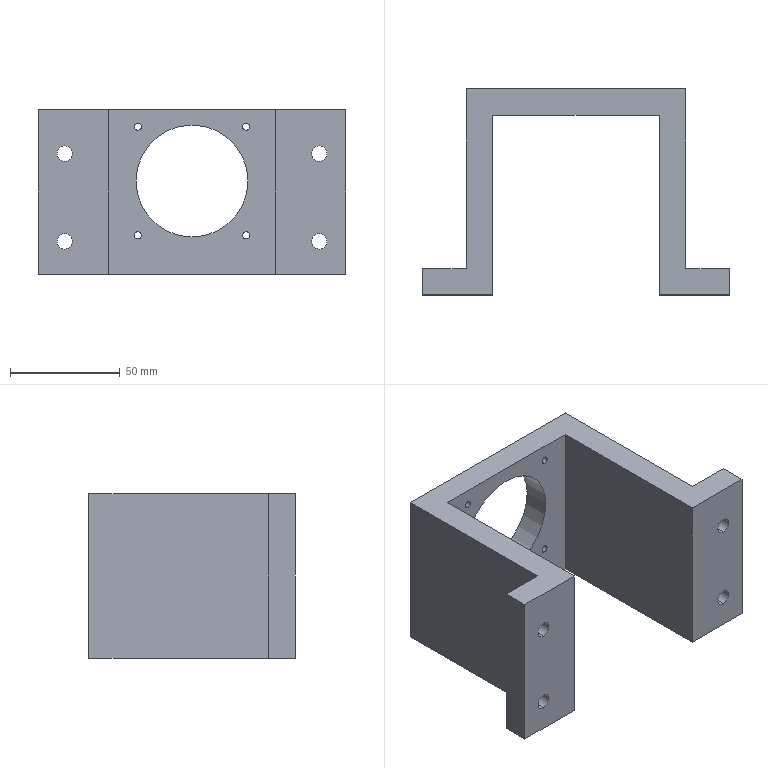Part | SolidWorks | features ICE 2, ExtruThin 1, HoleWzd 1 | 1 solid | 32 faces | box 140 x 94 x 75 mm | volume 246828 mm3 | cylinder 18 | plane 14 | commonest cylinder face diameters 3.3 x8 7 x8 51 x2
STEP:
#1=CARTESIAN_POINT('',(-24.749,70.,16.101));
#2=VERTEX_POINT('',#1);
#3=CARTESIAN_POINT('',(-24.749,70.,19.401));
#4=VERTEX_POINT('',#3);
#5=CARTESIAN_POINT('',(-24.749,70.,17.751));
#6=DIRECTION('',(0.,1.,0.));
#7=DIRECTION('',(0.,0.,1.));
#8=AXIS2_PLACEMENT_3D('',#5,#6,#7);
#9=CIRCLE('',#8,1.65);
#10=EDGE_CURVE('',#2,#4,#9,.T.);
#11=ORIENTED_EDGE('',*,*,#10,.F.);
#12=CARTESIAN_POINT('',(-24.749,82.,16.101));
#13=VERTEX_POINT('',#12);
#14=CARTESIAN_POINT('',(-24.749,82.,16.101));
#15=DIRECTION('',(0.,1.,0.));
#16=VECTOR('',#15,1000.);
#17=LINE('',#14,#16);
#18=EDGE_CURVE('',#2,#13,#17,.T.);
#19=ORIENTED_EDGE('',*,*,#18,.T.);
#20=CARTESIAN_POINT('',(-24.749,82.,19.401));
#21=VERTEX_POINT('',#20);
#22=CARTESIAN_POINT('',(-24.749,82.,17.751));
#23=DIRECTION('',(0.,1.,0.));
#24=DIRECTION('',(0.,0.,1.));
#25=AXIS2_PLACEMENT_3D('',#22,#23,#24);
#26=CIRCLE('',#25,1.65);
#27=EDGE_CURVE('',#13,#21,#26,.T.);
#28=ORIENTED_EDGE('',*,*,#27,.T.);
#29=CARTESIAN_POINT('',(-24.749,82.,19.401));
#30=DIRECTION('',(0.,1.,0.));
#31=VECTOR('',#30,1000.);
#32=LINE('',#29,#31);
#33=EDGE_CURVE('',#4,#21,#32,.T.);
#34=ORIENTED_EDGE('',*,*,#33,.F.);
#35=EDGE_LOOP('',(#11,#19,#28,#34));
#36=FACE_OUTER_BOUND('',#35,.T.);
#37=CARTESIAN_POINT('',(-24.749,82.,17.751));
#38=DIRECTION('',(0.,1.,0.));
#39=DIRECTION('',(0.,0.,1.));
#40=AXIS2_PLACEMENT_3D('',#37,#38,#39);
#41=CYLINDRICAL_SURFACE('',#40,1.65);
#42=ADVANCED_FACE('',(#36),#41,.F.);
#43=CARTESIAN_POINT('',(24.749,70.,16.101));
#44=VERTEX_POINT('',#43);
#45=CARTESIAN_POINT('',(24.749,70.,19.401));
#46=VERTEX_POINT('',#45);
#47=CARTESIAN_POINT('',(24.749,70.,17.751));
#48=DIRECTION('',(0.,1.,0.));
#49=DIRECTION('',(0.,0.,1.));
#50=AXIS2_PLACEMENT_3D('',#47,#48,#49);
#51=CIRCLE('',#50,1.65);
#52=EDGE_CURVE('',#44,#46,#51,.T.);
#53=ORIENTED_EDGE('',*,*,#52,.F.);
#54=CARTESIAN_POINT('',(24.749,82.,16.101));
#55=VERTEX_POINT('',#54);
#56=CARTESIAN_POINT('',(24.749,82.,16.101));
#57=DIRECTION('',(0.,1.,0.));
#58=VECTOR('',#57,1000.);
#59=LINE('',#56,#58);
#60=EDGE_CURVE('',#44,#55,#59,.T.);
#61=ORIENTED_EDGE('',*,*,#60,.T.);
#62=CARTESIAN_POINT('',(24.749,82.,19.401));
#63=VERTEX_POINT('',#62);
#64=CARTESIAN_POINT('',(24.749,82.,17.751));
#65=DIRECTION('',(0.,1.,0.));
#66=DIRECTION('',(0.,0.,1.));
#67=AXIS2_PLACEMENT_3D('',#64,#65,#66);
#68=CIRCLE('',#67,1.65);
#69=EDGE_CURVE('',#55,#63,#68,.T.);
#70=ORIENTED_EDGE('',*,*,#69,.T.);
#71=CARTESIAN_POINT('',(24.749,82.,19.401));
#72=DIRECTION('',(0.,1.,0.));
#73=VECTOR('',#72,1000.);
#74=LINE('',#71,#73);
#75=EDGE_CURVE('',#46,#63,#74,.T.);
#76=ORIENTED_EDGE('',*,*,#75,.F.);
#77=EDGE_LOOP('',(#53,#61,#70,#76));
#78=FACE_OUTER_BOUND('',#77,.T.);
#79=CARTESIAN_POINT('',(24.749,82.,17.751));
#80=DIRECTION('',(0.,1.,0.));
#81=DIRECTION('',(0.,0.,1.));
#82=AXIS2_PLACEMENT_3D('',#79,#80,#81);
#83=CYLINDRICAL_SURFACE('',#82,1.65);
#84=ADVANCED_FACE('',(#78),#83,.F.);
#85=CARTESIAN_POINT('',(24.749,70.,65.599));
#86=VERTEX_POINT('',#85);
#87=CARTESIAN_POINT('',(24.749,70.,68.899));
#88=VERTEX_POINT('',#87);
#89=CARTESIAN_POINT('',(24.749,70.,67.249));
#90=DIRECTION('',(0.,1.,0.));
#91=DIRECTION('',(0.,0.,1.));
#92=AXIS2_PLACEMENT_3D('',#89,#90,#91);
#93=CIRCLE('',#92,1.65);
#94=EDGE_CURVE('',#86,#88,#93,.T.);
#95=ORIENTED_EDGE('',*,*,#94,.F.);
#96=CARTESIAN_POINT('',(24.749,82.,65.599));
#97=VERTEX_POINT('',#96);
#98=CARTESIAN_POINT('',(24.749,82.,65.599));
#99=DIRECTION('',(0.,1.,0.));
#100=VECTOR('',#99,1000.);
#101=LINE('',#98,#100);
#102=EDGE_CURVE('',#86,#97,#101,.T.);
#103=ORIENTED_EDGE('',*,*,#102,.T.);
#104=CARTESIAN_POINT('',(24.749,82.,68.899));
#105=VERTEX_POINT('',#104);
#106=CARTESIAN_POINT('',(24.749,82.,67.249));
#107=DIRECTION('',(0.,1.,0.));
#108=DIRECTION('',(0.,0.,1.));
#109=AXIS2_PLACEMENT_3D('',#106,#107,#108);
#110=CIRCLE('',#109,1.65);
#111=EDGE_CURVE('',#97,#105,#110,.T.);
#112=ORIENTED_EDGE('',*,*,#111,.T.);
#113=CARTESIAN_POINT('',(24.749,82.,68.899));
#114=DIRECTION('',(0.,1.,0.));
#115=VECTOR('',#114,1000.);
#116=LINE('',#113,#115);
#117=EDGE_CURVE('',#88,#105,#116,.T.);
#118=ORIENTED_EDGE('',*,*,#117,.F.);
#119=EDGE_LOOP('',(#95,#103,#112,#118));
#120=FACE_OUTER_BOUND('',#119,.T.);
#121=CARTESIAN_POINT('',(24.749,82.,67.249));
#122=DIRECTION('',(0.,1.,0.));
#123=DIRECTION('',(0.,0.,1.));
#124=AXIS2_PLACEMENT_3D('',#121,#122,#123);
#125=CYLINDRICAL_SURFACE('',#124,1.65);
#126=ADVANCED_FACE('',(#120),#125,.F.);
#127=CARTESIAN_POINT('',(-24.749,70.,65.599));
#128=VERTEX_POINT('',#127);
#129=CARTESIAN_POINT('',(-24.749,70.,68.899));
#130=VERTEX_POINT('',#129);
#131=CARTESIAN_POINT('',(-24.749,70.,67.249));
#132=DIRECTION('',(0.,1.,0.));
#133=DIRECTION('',(0.,0.,1.));
#134=AXIS2_PLACEMENT_3D('',#131,#132,#133);
#135=CIRCLE('',#134,1.65);
#136=EDGE_CURVE('',#128,#130,#135,.T.);
#137=ORIENTED_EDGE('',*,*,#136,.F.);
#138=CARTESIAN_POINT('',(-24.749,82.,65.599));
#139=VERTEX_POINT('',#138);
#140=CARTESIAN_POINT('',(-24.749,82.,65.599));
#141=DIRECTION('',(0.,1.,0.));
#142=VECTOR('',#141,1000.);
#143=LINE('',#140,#142);
#144=EDGE_CURVE('',#128,#139,#143,.T.);
#145=ORIENTED_EDGE('',*,*,#144,.T.);
#146=CARTESIAN_POINT('',(-24.749,82.,68.899));
#147=VERTEX_POINT('',#146);
#148=CARTESIAN_POINT('',(-24.749,82.,67.249));
#149=DIRECTION('',(0.,1.,0.));
#150=DIRECTION('',(0.,0.,1.));
#151=AXIS2_PLACEMENT_3D('',#148,#149,#150);
#152=CIRCLE('',#151,1.65);
#153=EDGE_CURVE('',#139,#147,#152,.T.);
#154=ORIENTED_EDGE('',*,*,#153,.T.);
#155=CARTESIAN_POINT('',(-24.749,82.,68.899));
#156=DIRECTION('',(0.,1.,0.));
#157=VECTOR('',#156,1000.);
#158=LINE('',#155,#157);
#159=EDGE_CURVE('',#130,#147,#158,.T.);
#160=ORIENTED_EDGE('',*,*,#159,.F.);
#161=EDGE_LOOP('',(#137,#145,#154,#160));
#162=FACE_OUTER_BOUND('',#161,.T.);
#163=CARTESIAN_POINT('',(-24.749,82.,67.249));
#164=DIRECTION('',(0.,1.,0.));
#165=DIRECTION('',(0.,0.,1.));
#166=AXIS2_PLACEMENT_3D('',#163,#164,#165);
#167=CYLINDRICAL_SURFACE('',#166,1.65);
#168=ADVANCED_FACE('',(#162),#167,.F.);
#169=CARTESIAN_POINT('',(-58.,-12.,51.5));
#170=VERTEX_POINT('',#169);
#171=CARTESIAN_POINT('',(-58.,-12.,58.5));
#172=VERTEX_POINT('',#171);
#173=CARTESIAN_POINT('',(-58.,-12.,55.));
#174=DIRECTION('',(0.,1.,0.));
#175=DIRECTION('',(0.,0.,-1.));
#176=AXIS2_PLACEMENT_3D('',#173,#174,#175);
#177=CIRCLE('',#176,3.5);
#178=EDGE_CURVE('',#170,#172,#177,.T.);
#179=ORIENTED_EDGE('',*,*,#178,.F.);
#180=CARTESIAN_POINT('',(-58.,0.,51.5));
#181=VERTEX_POINT('',#180);
#182=CARTESIAN_POINT('',(-58.,-12.,51.5));
#183=DIRECTION('',(0.,1.,0.));
#184=VECTOR('',#183,1000.);
#185=LINE('',#182,#184);
#186=EDGE_CURVE('',#170,#181,#185,.T.);
#187=ORIENTED_EDGE('',*,*,#186,.T.);
#188=CARTESIAN_POINT('',(-58.,0.,58.5));
#189=VERTEX_POINT('',#188);
#190=CARTESIAN_POINT('',(-58.,0.,55.));
#191=DIRECTION('',(0.,1.,0.));
#192=DIRECTION('',(0.,0.,-1.));
#193=AXIS2_PLACEMENT_3D('',#190,#191,#192);
#194=CIRCLE('',#193,3.5);
#195=EDGE_CURVE('',#181,#189,#194,.T.);
#196=ORIENTED_EDGE('',*,*,#195,.T.);
#197=CARTESIAN_POINT('',(-58.,-12.,58.5));
#198=DIRECTION('',(0.,1.,0.));
#199=VECTOR('',#198,1000.);
#200=LINE('',#197,#199);
#201=EDGE_CURVE('',#172,#189,#200,.T.);
#202=ORIENTED_EDGE('',*,*,#201,.F.);
#203=EDGE_LOOP('',(#179,#187,#196,#202));
#204=FACE_OUTER_BOUND('',#203,.T.);
#205=CARTESIAN_POINT('',(-58.,-12.,55.));
#206=DIRECTION('',(0.,1.,0.));
#207=DIRECTION('',(0.,0.,1.));
#208=AXIS2_PLACEMENT_3D('',#205,#206,#207);
#209=CYLINDRICAL_SURFACE('',#208,3.5);
#210=ADVANCED_FACE('',(#204),#209,.F.);
#211=CARTESIAN_POINT('',(58.,-12.,51.5));
#212=VERTEX_POINT('',#211);
#213=CARTESIAN_POINT('',(58.,-12.,58.5));
#214=VERTEX_POINT('',#213);
#215=CARTESIAN_POINT('',(58.,-12.,55.));
#216=DIRECTION('',(0.,1.,0.));
#217=DIRECTION('',(0.,0.,1.));
#218=AXIS2_PLACEMENT_3D('',#215,#216,#217);
#219=CIRCLE('',#218,3.5);
#220=EDGE_CURVE('',#212,#214,#219,.T.);
#221=ORIENTED_EDGE('',*,*,#220,.F.);
#222=CARTESIAN_POINT('',(58.,0.,51.5));
#223=VERTEX_POINT('',#222);
#224=CARTESIAN_POINT('',(58.,-12.,51.5));
#225=DIRECTION('',(0.,1.,0.));
#226=VECTOR('',#225,1000.);
#227=LINE('',#224,#226);
#228=EDGE_CURVE('',#212,#223,#227,.T.);
#229=ORIENTED_EDGE('',*,*,#228,.T.);
#230=CARTESIAN_POINT('',(58.,0.,58.5));
#231=VERTEX_POINT('',#230);
#232=CARTESIAN_POINT('',(58.,0.,55.));
#233=DIRECTION('',(0.,1.,0.));
#234=DIRECTION('',(0.,0.,1.));
#235=AXIS2_PLACEMENT_3D('',#232,#233,#234);
#236=CIRCLE('',#235,3.5);
#237=EDGE_CURVE('',#223,#231,#236,.T.);
#238=ORIENTED_EDGE('',*,*,#237,.T.);
#239=CARTESIAN_POINT('',(58.,-12.,58.5));
#240=DIRECTION('',(0.,1.,0.));
#241=VECTOR('',#240,1000.);
#242=LINE('',#239,#241);
#243=EDGE_CURVE('',#214,#231,#242,.T.);
#244=ORIENTED_EDGE('',*,*,#243,.F.);
#245=EDGE_LOOP('',(#221,#229,#238,#244));
#246=FACE_OUTER_BOUND('',#245,.T.);
#247=CARTESIAN_POINT('',(58.,-12.,55.));
#248=DIRECTION('',(0.,1.,0.));
#249=DIRECTION('',(0.,0.,1.));
#250=AXIS2_PLACEMENT_3D('',#247,#248,#249);
#251=CYLINDRICAL_SURFACE('',#250,3.5);
#252=ADVANCED_FACE('',(#246),#251,.F.);
#253=CARTESIAN_POINT('',(58.,-12.,11.5));
#254=VERTEX_POINT('',#253);
#255=CARTESIAN_POINT('',(58.,-12.,18.5));
#256=VERTEX_POINT('',#255);
#257=CARTESIAN_POINT('',(58.,-12.,15.));
#258=DIRECTION('',(0.,1.,0.));
#259=DIRECTION('',(0.,0.,-1.));
#260=AXIS2_PLACEMENT_3D('',#257,#258,#259);
#261=CIRCLE('',#260,3.5);
#262=EDGE_CURVE('',#254,#256,#261,.T.);
#263=ORIENTED_EDGE('',*,*,#262,.F.);
#264=CARTESIAN_POINT('',(58.,0.,11.5));
#265=VERTEX_POINT('',#264);
#266=CARTESIAN_POINT('',(58.,-12.,11.5));
#267=DIRECTION('',(0.,1.,0.));
#268=VECTOR('',#267,1000.);
#269=LINE('',#266,#268);
#270=EDGE_CURVE('',#254,#265,#269,.T.);
#271=ORIENTED_EDGE('',*,*,#270,.T.);
#272=CARTESIAN_POINT('',(58.,0.,18.5));
#273=VERTEX_POINT('',#272);
#274=CARTESIAN_POINT('',(58.,0.,15.));
#275=DIRECTION('',(0.,1.,0.));
#276=DIRECTION('',(0.,0.,-1.));
#277=AXIS2_PLACEMENT_3D('',#274,#275,#276);
#278=CIRCLE('',#277,3.5);
#279=EDGE_CURVE('',#265,#273,#278,.T.);
#280=ORIENTED_EDGE('',*,*,#279,.T.);
#281=CARTESIAN_POINT('',(58.,-12.,18.5));
#282=DIRECTION('',(0.,1.,0.));
#283=VECTOR('',#282,1000.);
#284=LINE('',#281,#283);
#285=EDGE_CURVE('',#256,#273,#284,.T.);
#286=ORIENTED_EDGE('',*,*,#285,.F.);
#287=EDGE_LOOP('',(#263,#271,#280,#286));
#288=FACE_OUTER_BOUND('',#287,.T.);
#289=CARTESIAN_POINT('',(58.,-12.,15.));
#290=DIRECTION('',(0.,1.,0.));
#291=DIRECTION('',(0.,0.,1.));
#292=AXIS2_PLACEMENT_3D('',#289,#290,#291);
#293=CYLINDRICAL_SURFACE('',#292,3.5);
#294=ADVANCED_FACE('',(#288),#293,.F.);
#295=CARTESIAN_POINT('',(-58.,-12.,11.5));
#296=VERTEX_POINT('',#295);
#297=CARTESIAN_POINT('',(-58.,-12.,18.5));
#298=VERTEX_POINT('',#297);
#299=CARTESIAN_POINT('',(-58.,-12.,15.));
#300=DIRECTION('',(0.,1.,0.));
#301=DIRECTION('',(0.,0.,1.));
#302=AXIS2_PLACEMENT_3D('',#299,#300,#301);
#303=CIRCLE('',#302,3.5);
#304=EDGE_CURVE('',#296,#298,#303,.T.);
#305=ORIENTED_EDGE('',*,*,#304,.F.);
#306=CARTESIAN_POINT('',(-58.,0.,11.5));
#307=VERTEX_POINT('',#306);
#308=CARTESIAN_POINT('',(-58.,-12.,11.5));
#309=DIRECTION('',(0.,1.,0.));
#310=VECTOR('',#309,1000.);
#311=LINE('',#308,#310);
#312=EDGE_CURVE('',#296,#307,#311,.T.);
#313=ORIENTED_EDGE('',*,*,#312,.T.);
#314=CARTESIAN_POINT('',(-58.,0.,18.5));
#315=VERTEX_POINT('',#314);
#316=CARTESIAN_POINT('',(-58.,0.,15.));
#317=DIRECTION('',(0.,1.,0.));
#318=DIRECTION('',(0.,0.,1.));
#319=AXIS2_PLACEMENT_3D('',#316,#317,#318);
#320=CIRCLE('',#319,3.5);
#321=EDGE_CURVE('',#307,#315,#320,.T.);
#322=ORIENTED_EDGE('',*,*,#321,.T.);
#323=CARTESIAN_POINT('',(-58.,-12.,18.5));
#324=DIRECTION('',(0.,1.,0.));
#325=VECTOR('',#324,1000.);
#326=LINE('',#323,#325);
#327=EDGE_CURVE('',#298,#315,#326,.T.);
#328=ORIENTED_EDGE('',*,*,#327,.F.);
#329=EDGE_LOOP('',(#305,#313,#322,#328));
#330=FACE_OUTER_BOUND('',#329,.T.);
#331=CARTESIAN_POINT('',(-58.,-12.,15.));
#332=DIRECTION('',(0.,1.,0.));
#333=DIRECTION('',(0.,0.,1.));
#334=AXIS2_PLACEMENT_3D('',#331,#332,#333);
#335=CYLINDRICAL_SURFACE('',#334,3.5);
#336=ADVANCED_FACE('',(#330),#335,.F.);
#337=CARTESIAN_POINT('',(0.,70.,17.));
#338=VERTEX_POINT('',#337);
#339=CARTESIAN_POINT('',(0.,70.,68.));
#340=VERTEX_POINT('',#339);
#341=CARTESIAN_POINT('',(0.,70.,42.5));
#342=DIRECTION('',(0.,1.,0.));
#343=DIRECTION('',(0.,0.,1.));
#344=AXIS2_PLACEMENT_3D('',#341,#342,#343);
#345=CIRCLE('',#344,25.5);
#346=EDGE_CURVE('',#338,#340,#345,.T.);
#347=ORIENTED_EDGE('',*,*,#346,.F.);
#348=CARTESIAN_POINT('',(0.,82.,17.));
#349=VERTEX_POINT('',#348);
#350=CARTESIAN_POINT('',(0.,-12.,17.));
#351=DIRECTION('',(0.,1.,0.));
#352=VECTOR('',#351,1000.);
#353=LINE('',#350,#352);
#354=EDGE_CURVE('',#338,#349,#353,.T.);
#355=ORIENTED_EDGE('',*,*,#354,.T.);
#356=CARTESIAN_POINT('',(0.,82.,68.));
#357=VERTEX_POINT('',#356);
#358=CARTESIAN_POINT('',(0.,82.,42.5));
#359=DIRECTION('',(0.,1.,0.));
#360=DIRECTION('',(0.,0.,1.));
#361=AXIS2_PLACEMENT_3D('',#358,#359,#360);
#362=CIRCLE('',#361,25.5);
#363=EDGE_CURVE('',#349,#357,#362,.T.);
#364=ORIENTED_EDGE('',*,*,#363,.T.);
#365=CARTESIAN_POINT('',(0.,-12.,68.));
#366=DIRECTION('',(0.,1.,0.));
#367=VECTOR('',#366,1000.);
#368=LINE('',#365,#367);
#369=EDGE_CURVE('',#340,#357,#368,.T.);
#370=ORIENTED_EDGE('',*,*,#369,.F.);
#371=EDGE_LOOP('',(#347,#355,#364,#370));
#372=FACE_OUTER_BOUND('',#371,.T.);
#373=CARTESIAN_POINT('',(0.,-12.,42.5));
#374=DIRECTION('',(0.,1.,0.));
#375=DIRECTION('',(0.,0.,1.));
#376=AXIS2_PLACEMENT_3D('',#373,#374,#375);
#377=CYLINDRICAL_SURFACE('',#376,25.5);
#378=ADVANCED_FACE('',(#372),#377,.F.);
#379=CARTESIAN_POINT('',(58.,-12.,55.));
#380=DIRECTION('',(0.,1.,0.));
#381=DIRECTION('',(0.,0.,1.));
#382=AXIS2_PLACEMENT_3D('',#379,#380,#381);
#383=CIRCLE('',#382,3.5);
#384=EDGE_CURVE('',#214,#212,#383,.T.);
#385=ORIENTED_EDGE('',*,*,#384,.T.);
#386=ORIENTED_EDGE('',*,*,#220,.T.);
#387=EDGE_LOOP('',(#385,#386));
#388=FACE_BOUND('',#387,.T.);
#389=CARTESIAN_POINT('',(58.,-12.,15.));
#390=DIRECTION('',(0.,1.,0.));
#391=DIRECTION('',(0.,0.,-1.));
#392=AXIS2_PLACEMENT_3D('',#389,#390,#391);
#393=CIRCLE('',#392,3.5);
#394=EDGE_CURVE('',#256,#254,#393,.T.);
#395=ORIENTED_EDGE('',*,*,#394,.T.);
#396=ORIENTED_EDGE('',*,*,#262,.T.);
#397=EDGE_LOOP('',(#395,#396));
#398=FACE_BOUND('',#397,.T.);
#399=CARTESIAN_POINT('',(38.,-12.,0.));
#400=VERTEX_POINT('',#399);
#401=CARTESIAN_POINT('',(70.,-12.,0.));
#402=VERTEX_POINT('',#401);
#403=CARTESIAN_POINT('',(50.,-12.,0.));
#404=DIRECTION('',(1.,0.,0.));
#405=VECTOR('',#404,1000.);
#406=LINE('',#403,#405);
#407=EDGE_CURVE('',#400,#402,#406,.T.);
#408=ORIENTED_EDGE('',*,*,#407,.T.);
#409=CARTESIAN_POINT('',(70.,-12.,75.));
#410=VERTEX_POINT('',#409);
#411=CARTESIAN_POINT('',(70.,-12.,75.));
#412=DIRECTION('',(0.,0.,-1.));
#413=VECTOR('',#412,1000.);
#414=LINE('',#411,#413);
#415=EDGE_CURVE('',#410,#402,#414,.T.);
#416=ORIENTED_EDGE('',*,*,#415,.F.);
#417=CARTESIAN_POINT('',(38.,-12.,75.));
#418=VERTEX_POINT('',#417);
#419=CARTESIAN_POINT('',(50.,-12.,75.));
#420=DIRECTION('',(1.,0.,0.));
#421=VECTOR('',#420,1000.);
#422=LINE('',#419,#421);
#423=EDGE_CURVE('',#418,#410,#422,.T.);
#424=ORIENTED_EDGE('',*,*,#423,.F.);
#425=CARTESIAN_POINT('',(38.,-12.,75.));
#426=DIRECTION('',(0.,0.,-1.));
#427=VECTOR('',#426,1000.);
#428=LINE('',#425,#427);
#429=EDGE_CURVE('',#418,#400,#428,.T.);
#430=ORIENTED_EDGE('',*,*,#429,.T.);
#431=EDGE_LOOP('',(#408,#416,#424,#430));
#432=FACE_OUTER_BOUND('',#431,.T.);
#433=CARTESIAN_POINT('',(50.,-12.,75.));
#434=DIRECTION('',(0.,1.,0.));
#435=DIRECTION('',(0.,0.,1.));
#436=AXIS2_PLACEMENT_3D('',#433,#434,#435);
#437=PLANE('',#436);
#438=ADVANCED_FACE('',(#388,#398,#432),#437,.F.);
#439=CARTESIAN_POINT('',(70.,0.,0.));
#440=VERTEX_POINT('',#439);
#441=CARTESIAN_POINT('',(70.,0.,0.));
#442=DIRECTION('',(0.,-1.,0.));
#443=VECTOR('',#442,1000.);
#444=LINE('',#441,#443);
#445=EDGE_CURVE('',#440,#402,#444,.T.);
#446=ORIENTED_EDGE('',*,*,#445,.F.);
#447=CARTESIAN_POINT('',(70.,0.,75.));
#448=VERTEX_POINT('',#447);
#449=CARTESIAN_POINT('',(70.,0.,75.));
#450=DIRECTION('',(0.,0.,-1.));
#451=VECTOR('',#450,1000.);
#452=LINE('',#449,#451);
#453=EDGE_CURVE('',#448,#440,#452,.T.);
#454=ORIENTED_EDGE('',*,*,#453,.F.);
#455=CARTESIAN_POINT('',(70.,0.,75.));
#456=DIRECTION('',(0.,-1.,0.));
#457=VECTOR('',#456,1000.);
#458=LINE('',#455,#457);
#459=EDGE_CURVE('',#448,#410,#458,.T.);
#460=ORIENTED_EDGE('',*,*,#459,.T.);
#461=ORIENTED_EDGE('',*,*,#415,.T.);
#462=EDGE_LOOP('',(#446,#454,#460,#461));
#463=FACE_OUTER_BOUND('',#462,.T.);
#464=CARTESIAN_POINT('',(70.,0.,75.));
#465=DIRECTION('',(1.,0.,0.));
#466=DIRECTION('',(0.,0.,-1.));
#467=AXIS2_PLACEMENT_3D('',#464,#465,#466);
#468=PLANE('',#467);
#469=ADVANCED_FACE('',(#463),#468,.T.);
#470=CARTESIAN_POINT('',(58.,0.,55.));
#471=DIRECTION('',(0.,1.,0.));
#472=DIRECTION('',(0.,0.,1.));
#473=AXIS2_PLACEMENT_3D('',#470,#471,#472);
#474=CIRCLE('',#473,3.5);
#475=EDGE_CURVE('',#231,#223,#474,.T.);
#476=ORIENTED_EDGE('',*,*,#475,.F.);
#477=ORIENTED_EDGE('',*,*,#237,.F.);
#478=EDGE_LOOP('',(#476,#477));
#479=FACE_BOUND('',#478,.T.);
#480=CARTESIAN_POINT('',(58.,0.,15.));
#481=DIRECTION('',(0.,1.,0.));
#482=DIRECTION('',(0.,0.,-1.));
#483=AXIS2_PLACEMENT_3D('',#480,#481,#482);
#484=CIRCLE('',#483,3.5);
#485=EDGE_CURVE('',#273,#265,#484,.T.);
#486=ORIENTED_EDGE('',*,*,#485,.F.);
#487=ORIENTED_EDGE('',*,*,#279,.F.);
#488=EDGE_LOOP('',(#486,#487));
#489=FACE_BOUND('',#488,.T.);
#490=CARTESIAN_POINT('',(50.,0.,0.));
#491=VERTEX_POINT('',#490);
#492=CARTESIAN_POINT('',(50.,0.,0.));
#493=DIRECTION('',(1.,0.,0.));
#494=VECTOR('',#493,1000.);
#495=LINE('',#492,#494);
#496=EDGE_CURVE('',#491,#440,#495,.T.);
#497=ORIENTED_EDGE('',*,*,#496,.F.);
#498=CARTESIAN_POINT('',(50.,0.,75.));
#499=VERTEX_POINT('',#498);
#500=CARTESIAN_POINT('',(50.,0.,75.));
#501=DIRECTION('',(0.,0.,-1.));
#502=VECTOR('',#501,1000.);
#503=LINE('',#500,#502);
#504=EDGE_CURVE('',#499,#491,#503,.T.);
#505=ORIENTED_EDGE('',*,*,#504,.F.);
#506=CARTESIAN_POINT('',(50.,0.,75.));
#507=DIRECTION('',(1.,0.,0.));
#508=VECTOR('',#507,1000.);
#509=LINE('',#506,#508);
#510=EDGE_CURVE('',#499,#448,#509,.T.);
#511=ORIENTED_EDGE('',*,*,#510,.T.);
#512=ORIENTED_EDGE('',*,*,#453,.T.);
#513=EDGE_LOOP('',(#497,#505,#511,#512));
#514=FACE_OUTER_BOUND('',#513,.T.);
#515=CARTESIAN_POINT('',(50.,0.,75.));
#516=DIRECTION('',(0.,1.,0.));
#517=DIRECTION('',(0.,0.,1.));
#518=AXIS2_PLACEMENT_3D('',#515,#516,#517);
#519=PLANE('',#518);
#520=ADVANCED_FACE('',(#479,#489,#514),#519,.T.);
#521=CARTESIAN_POINT('',(50.,82.,0.));
#522=VERTEX_POINT('',#521);
#523=CARTESIAN_POINT('',(50.,82.,0.));
#524=DIRECTION('',(0.,-1.,0.));
#525=VECTOR('',#524,1000.);
#526=LINE('',#523,#525);
#527=EDGE_CURVE('',#522,#491,#526,.T.);
#528=ORIENTED_EDGE('',*,*,#527,.F.);
#529=CARTESIAN_POINT('',(50.,82.,75.));
#530=VERTEX_POINT('',#529);
#531=CARTESIAN_POINT('',(50.,82.,75.));
#532=DIRECTION('',(0.,0.,-1.));
#533=VECTOR('',#532,1000.);
#534=LINE('',#531,#533);
#535=EDGE_CURVE('',#530,#522,#534,.T.);
#536=ORIENTED_EDGE('',*,*,#535,.F.);
#537=CARTESIAN_POINT('',(50.,82.,75.));
#538=DIRECTION('',(0.,-1.,0.));
#539=VECTOR('',#538,1000.);
#540=LINE('',#537,#539);
#541=EDGE_CURVE('',#530,#499,#540,.T.);
#542=ORIENTED_EDGE('',*,*,#541,.T.);
#543=ORIENTED_EDGE('',*,*,#504,.T.);
#544=EDGE_LOOP('',(#528,#536,#542,#543));
#545=FACE_OUTER_BOUND('',#544,.T.);
#546=CARTESIAN_POINT('',(50.,82.,75.));
#547=DIRECTION('',(1.,0.,0.));
#548=DIRECTION('',(0.,0.,-1.));
#549=AXIS2_PLACEMENT_3D('',#546,#547,#548);
#550=PLANE('',#549);
#551=ADVANCED_FACE('',(#545),#550,.T.);
#552=CARTESIAN_POINT('',(-24.749,82.,17.751));
#553=DIRECTION('',(0.,1.,0.));
#554=DIRECTION('',(0.,0.,1.));
#555=AXIS2_PLACEMENT_3D('',#552,#553,#554);
#556=CIRCLE('',#555,1.65);
#557=EDGE_CURVE('',#21,#13,#556,.T.);
#558=ORIENTED_EDGE('',*,*,#557,.F.);
#559=ORIENTED_EDGE('',*,*,#27,.F.);
#560=EDGE_LOOP('',(#558,#559));
#561=FACE_BOUND('',#560,.T.);
#562=CARTESIAN_POINT('',(24.749,82.,17.751));
#563=DIRECTION('',(0.,1.,0.));
#564=DIRECTION('',(0.,0.,1.));
#565=AXIS2_PLACEMENT_3D('',#562,#563,#564);
#566=CIRCLE('',#565,1.65);
#567=EDGE_CURVE('',#63,#55,#566,.T.);
#568=ORIENTED_EDGE('',*,*,#567,.F.);
#569=ORIENTED_EDGE('',*,*,#69,.F.);
#570=EDGE_LOOP('',(#568,#569));
#571=FACE_BOUND('',#570,.T.);
#572=CARTESIAN_POINT('',(24.749,82.,67.249));
#573=DIRECTION('',(0.,1.,0.));
#574=DIRECTION('',(0.,0.,1.));
#575=AXIS2_PLACEMENT_3D('',#572,#573,#574);
#576=CIRCLE('',#575,1.65);
#577=EDGE_CURVE('',#105,#97,#576,.T.);
#578=ORIENTED_EDGE('',*,*,#577,.F.);
#579=ORIENTED_EDGE('',*,*,#111,.F.);
#580=EDGE_LOOP('',(#578,#579));
#581=FACE_BOUND('',#580,.T.);
#582=CARTESIAN_POINT('',(-24.749,82.,67.249));
#583=DIRECTION('',(0.,1.,0.));
#584=DIRECTION('',(0.,0.,1.));
#585=AXIS2_PLACEMENT_3D('',#582,#583,#584);
#586=CIRCLE('',#585,1.65);
#587=EDGE_CURVE('',#147,#139,#586,.T.);
#588=ORIENTED_EDGE('',*,*,#587,.F.);
#589=ORIENTED_EDGE('',*,*,#153,.F.);
#590=EDGE_LOOP('',(#588,#589));
#591=FACE_BOUND('',#590,.T.);
#592=CARTESIAN_POINT('',(0.,82.,42.5));
#593=DIRECTION('',(0.,1.,0.));
#594=DIRECTION('',(0.,0.,1.));
#595=AXIS2_PLACEMENT_3D('',#592,#593,#594);
#596=CIRCLE('',#595,25.5);
#597=EDGE_CURVE('',#357,#349,#596,.T.);
#598=ORIENTED_EDGE('',*,*,#597,.F.);
#599=ORIENTED_EDGE('',*,*,#363,.F.);
#600=EDGE_LOOP('',(#598,#599));
#601=FACE_BOUND('',#600,.T.);
#602=CARTESIAN_POINT('',(-50.,82.,0.));
#603=VERTEX_POINT('',#602);
#604=CARTESIAN_POINT('',(-50.,82.,0.));
#605=DIRECTION('',(1.,0.,0.));
#606=VECTOR('',#605,1000.);
#607=LINE('',#604,#606);
#608=EDGE_CURVE('',#603,#522,#607,.T.);
#609=ORIENTED_EDGE('',*,*,#608,.F.);
#610=CARTESIAN_POINT('',(-50.,82.,75.));
#611=VERTEX_POINT('',#610);
#612=CARTESIAN_POINT('',(-50.,82.,75.));
#613=DIRECTION('',(0.,0.,-1.));
#614=VECTOR('',#613,1000.);
#615=LINE('',#612,#614);
#616=EDGE_CURVE('',#611,#603,#615,.T.);
#617=ORIENTED_EDGE('',*,*,#616,.F.);
#618=CARTESIAN_POINT('',(-50.,82.,75.));
#619=DIRECTION('',(1.,0.,0.));
#620=VECTOR('',#619,1000.);
#621=LINE('',#618,#620);
#622=EDGE_CURVE('',#611,#530,#621,.T.);
#623=ORIENTED_EDGE('',*,*,#622,.T.);
#624=ORIENTED_EDGE('',*,*,#535,.T.);
#625=EDGE_LOOP('',(#609,#617,#623,#624));
#626=FACE_OUTER_BOUND('',#625,.T.);
#627=CARTESIAN_POINT('',(-50.,82.,75.));
#628=DIRECTION('',(0.,1.,0.));
#629=DIRECTION('',(0.,0.,1.));
#630=AXIS2_PLACEMENT_3D('',#627,#628,#629);
#631=PLANE('',#630);
#632=ADVANCED_FACE('',(#561,#571,#581,#591,#601,#626),#631,.T.);
#633=CARTESIAN_POINT('',(-50.,0.,0.));
#634=VERTEX_POINT('',#633);
#635=CARTESIAN_POINT('',(-50.,0.,0.));
#636=DIRECTION('',(0.,1.,0.));
#637=VECTOR('',#636,1000.);
#638=LINE('',#635,#637);
#639=EDGE_CURVE('',#634,#603,#638,.T.);
#640=ORIENTED_EDGE('',*,*,#639,.F.);
#641=CARTESIAN_POINT('',(-50.,0.,75.));
#642=VERTEX_POINT('',#641);
#643=CARTESIAN_POINT('',(-50.,0.,75.));
#644=DIRECTION('',(0.,0.,-1.));
#645=VECTOR('',#644,1000.);
#646=LINE('',#643,#645);
#647=EDGE_CURVE('',#642,#634,#646,.T.);
#648=ORIENTED_EDGE('',*,*,#647,.F.);
#649=CARTESIAN_POINT('',(-50.,0.,75.));
#650=DIRECTION('',(0.,1.,0.));
#651=VECTOR('',#650,1000.);
#652=LINE('',#649,#651);
#653=EDGE_CURVE('',#642,#611,#652,.T.);
#654=ORIENTED_EDGE('',*,*,#653,.T.);
#655=ORIENTED_EDGE('',*,*,#616,.T.);
#656=EDGE_LOOP('',(#640,#648,#654,#655));
#657=FACE_OUTER_BOUND('',#656,.T.);
#658=CARTESIAN_POINT('',(-50.,0.,75.));
#659=DIRECTION('',(-1.,0.,0.));
#660=DIRECTION('',(0.,0.,1.));
#661=AXIS2_PLACEMENT_3D('',#658,#659,#660);
#662=PLANE('',#661);
#663=ADVANCED_FACE('',(#657),#662,.T.);
#664=CARTESIAN_POINT('',(-58.,0.,55.));
#665=DIRECTION('',(0.,1.,0.));
#666=DIRECTION('',(0.,0.,-1.));
#667=AXIS2_PLACEMENT_3D('',#664,#665,#666);
#668=CIRCLE('',#667,3.5);
#669=EDGE_CURVE('',#189,#181,#668,.T.);
#670=ORIENTED_EDGE('',*,*,#669,.F.);
#671=ORIENTED_EDGE('',*,*,#195,.F.);
#672=EDGE_LOOP('',(#670,#671));
#673=FACE_BOUND('',#672,.T.);
#674=CARTESIAN_POINT('',(-58.,0.,15.));
#675=DIRECTION('',(0.,1.,0.));
#676=DIRECTION('',(0.,0.,1.));
#677=AXIS2_PLACEMENT_3D('',#674,#675,#676);
#678=CIRCLE('',#677,3.5);
#679=EDGE_CURVE('',#315,#307,#678,.T.);
#680=ORIENTED_EDGE('',*,*,#679,.F.);
#681=ORIENTED_EDGE('',*,*,#321,.F.);
#682=EDGE_LOOP('',(#680,#681));
#683=FACE_BOUND('',#682,.T.);
#684=CARTESIAN_POINT('',(-70.,0.,0.));
#685=VERTEX_POINT('',#684);
#686=CARTESIAN_POINT('',(-70.,0.,0.));
#687=DIRECTION('',(1.,0.,0.));
#688=VECTOR('',#687,1000.);
#689=LINE('',#686,#688);
#690=EDGE_CURVE('',#685,#634,#689,.T.);
#691=ORIENTED_EDGE('',*,*,#690,.F.);
#692=CARTESIAN_POINT('',(-70.,0.,75.));
#693=VERTEX_POINT('',#692);
#694=CARTESIAN_POINT('',(-70.,0.,75.));
#695=DIRECTION('',(0.,0.,-1.));
#696=VECTOR('',#695,1000.);
#697=LINE('',#694,#696);
#698=EDGE_CURVE('',#693,#685,#697,.T.);
#699=ORIENTED_EDGE('',*,*,#698,.F.);
#700=CARTESIAN_POINT('',(-70.,0.,75.));
#701=DIRECTION('',(1.,0.,0.));
#702=VECTOR('',#701,1000.);
#703=LINE('',#700,#702);
#704=EDGE_CURVE('',#693,#642,#703,.T.);
#705=ORIENTED_EDGE('',*,*,#704,.T.);
#706=ORIENTED_EDGE('',*,*,#647,.T.);
#707=EDGE_LOOP('',(#691,#699,#705,#706));
#708=FACE_OUTER_BOUND('',#707,.T.);
#709=CARTESIAN_POINT('',(-70.,0.,75.));
#710=DIRECTION('',(0.,1.,0.));
#711=DIRECTION('',(0.,0.,1.));
#712=AXIS2_PLACEMENT_3D('',#709,#710,#711);
#713=PLANE('',#712);
#714=ADVANCED_FACE('',(#673,#683,#708),#713,.T.);
#715=CARTESIAN_POINT('',(-70.,-12.,0.));
#716=VERTEX_POINT('',#715);
#717=CARTESIAN_POINT('',(-70.,-12.,0.));
#718=DIRECTION('',(0.,1.,0.));
#719=VECTOR('',#718,1000.);
#720=LINE('',#717,#719);
#721=EDGE_CURVE('',#716,#685,#720,.T.);
#722=ORIENTED_EDGE('',*,*,#721,.F.);
#723=CARTESIAN_POINT('',(-70.,-12.,75.));
#724=VERTEX_POINT('',#723);
#725=CARTESIAN_POINT('',(-70.,-12.,75.));
#726=DIRECTION('',(0.,0.,-1.));
#727=VECTOR('',#726,1000.);
#728=LINE('',#725,#727);
#729=EDGE_CURVE('',#724,#716,#728,.T.);
#730=ORIENTED_EDGE('',*,*,#729,.F.);
#731=CARTESIAN_POINT('',(-70.,-12.,75.));
#732=DIRECTION('',(0.,1.,0.));
#733=VECTOR('',#732,1000.);
#734=LINE('',#731,#733);
#735=EDGE_CURVE('',#724,#693,#734,.T.);
#736=ORIENTED_EDGE('',*,*,#735,.T.);
#737=ORIENTED_EDGE('',*,*,#698,.T.);
#738=EDGE_LOOP('',(#722,#730,#736,#737));
#739=FACE_OUTER_BOUND('',#738,.T.);
#740=CARTESIAN_POINT('',(-70.,-12.,75.));
#741=DIRECTION('',(-1.,0.,0.));
#742=DIRECTION('',(0.,0.,1.));
#743=AXIS2_PLACEMENT_3D('',#740,#741,#742);
#744=PLANE('',#743);
#745=ADVANCED_FACE('',(#739),#744,.T.);
#746=CARTESIAN_POINT('',(-58.,-12.,55.));
#747=DIRECTION('',(0.,1.,0.));
#748=DIRECTION('',(0.,0.,-1.));
#749=AXIS2_PLACEMENT_3D('',#746,#747,#748);
#750=CIRCLE('',#749,3.5);
#751=EDGE_CURVE('',#172,#170,#750,.T.);
#752=ORIENTED_EDGE('',*,*,#751,.T.);
#753=ORIENTED_EDGE('',*,*,#178,.T.);
#754=EDGE_LOOP('',(#752,#753));
#755=FACE_BOUND('',#754,.T.);
#756=CARTESIAN_POINT('',(-58.,-12.,15.));
#757=DIRECTION('',(0.,1.,0.));
#758=DIRECTION('',(0.,0.,1.));
#759=AXIS2_PLACEMENT_3D('',#756,#757,#758);
#760=CIRCLE('',#759,3.5);
#761=EDGE_CURVE('',#298,#296,#760,.T.);
#762=ORIENTED_EDGE('',*,*,#761,.T.);
#763=ORIENTED_EDGE('',*,*,#304,.T.);
#764=EDGE_LOOP('',(#762,#763));
#765=FACE_BOUND('',#764,.T.);
#766=CARTESIAN_POINT('',(-38.,-12.,0.));
#767=VERTEX_POINT('',#766);
#768=CARTESIAN_POINT('',(-70.,-12.,0.));
#769=DIRECTION('',(1.,0.,0.));
#770=VECTOR('',#769,1000.);
#771=LINE('',#768,#770);
#772=EDGE_CURVE('',#716,#767,#771,.T.);
#773=ORIENTED_EDGE('',*,*,#772,.T.);
#774=CARTESIAN_POINT('',(-38.,-12.,75.));
#775=VERTEX_POINT('',#774);
#776=CARTESIAN_POINT('',(-38.,-12.,75.));
#777=DIRECTION('',(0.,0.,-1.));
#778=VECTOR('',#777,1000.);
#779=LINE('',#776,#778);
#780=EDGE_CURVE('',#775,#767,#779,.T.);
#781=ORIENTED_EDGE('',*,*,#780,.F.);
#782=CARTESIAN_POINT('',(-70.,-12.,75.));
#783=DIRECTION('',(1.,0.,0.));
#784=VECTOR('',#783,1000.);
#785=LINE('',#782,#784);
#786=EDGE_CURVE('',#724,#775,#785,.T.);
#787=ORIENTED_EDGE('',*,*,#786,.F.);
#788=ORIENTED_EDGE('',*,*,#729,.T.);
#789=EDGE_LOOP('',(#773,#781,#787,#788));
#790=FACE_OUTER_BOUND('',#789,.T.);
#791=CARTESIAN_POINT('',(-70.,-12.,75.));
#792=DIRECTION('',(0.,1.,0.));
#793=DIRECTION('',(0.,0.,1.));
#794=AXIS2_PLACEMENT_3D('',#791,#792,#793);
#795=PLANE('',#794);
#796=ADVANCED_FACE('',(#755,#765,#790),#795,.F.);
#797=CARTESIAN_POINT('',(-38.,70.,0.));
#798=VERTEX_POINT('',#797);
#799=CARTESIAN_POINT('',(-38.,0.,0.));
#800=DIRECTION('',(0.,1.,0.));
#801=VECTOR('',#800,1000.);
#802=LINE('',#799,#801);
#803=EDGE_CURVE('',#767,#798,#802,.T.);
#804=ORIENTED_EDGE('',*,*,#803,.T.);
#805=CARTESIAN_POINT('',(-38.,70.,75.));
#806=VERTEX_POINT('',#805);
#807=CARTESIAN_POINT('',(-38.,70.,75.));
#808=DIRECTION('',(0.,0.,-1.));
#809=VECTOR('',#808,1000.);
#810=LINE('',#807,#809);
#811=EDGE_CURVE('',#806,#798,#810,.T.);
#812=ORIENTED_EDGE('',*,*,#811,.F.);
#813=CARTESIAN_POINT('',(-38.,0.,75.));
#814=DIRECTION('',(0.,1.,0.));
#815=VECTOR('',#814,1000.);
#816=LINE('',#813,#815);
#817=EDGE_CURVE('',#775,#806,#816,.T.);
#818=ORIENTED_EDGE('',*,*,#817,.F.);
#819=ORIENTED_EDGE('',*,*,#780,.T.);
#820=EDGE_LOOP('',(#804,#812,#818,#819));
#821=FACE_OUTER_BOUND('',#820,.T.);
#822=CARTESIAN_POINT('',(-38.,0.,75.));
#823=DIRECTION('',(-1.,0.,0.));
#824=DIRECTION('',(0.,0.,1.));
#825=AXIS2_PLACEMENT_3D('',#822,#823,#824);
#826=PLANE('',#825);
#827=ADVANCED_FACE('',(#821),#826,.F.);
#828=CARTESIAN_POINT('',(-24.749,70.,17.751));
#829=DIRECTION('',(0.,1.,0.));
#830=DIRECTION('',(0.,0.,1.));
#831=AXIS2_PLACEMENT_3D('',#828,#829,#830);
#832=CIRCLE('',#831,1.65);
#833=EDGE_CURVE('',#4,#2,#832,.T.);
#834=ORIENTED_EDGE('',*,*,#833,.T.);
#835=ORIENTED_EDGE('',*,*,#10,.T.);
#836=EDGE_LOOP('',(#834,#835));
#837=FACE_BOUND('',#836,.T.);
#838=CARTESIAN_POINT('',(24.749,70.,17.751));
#839=DIRECTION('',(0.,1.,0.));
#840=DIRECTION('',(0.,0.,1.));
#841=AXIS2_PLACEMENT_3D('',#838,#839,#840);
#842=CIRCLE('',#841,1.65);
#843=EDGE_CURVE('',#46,#44,#842,.T.);
#844=ORIENTED_EDGE('',*,*,#843,.T.);
#845=ORIENTED_EDGE('',*,*,#52,.T.);
#846=EDGE_LOOP('',(#844,#845));
#847=FACE_BOUND('',#846,.T.);
#848=CARTESIAN_POINT('',(24.749,70.,67.249));
#849=DIRECTION('',(0.,1.,0.));
#850=DIRECTION('',(0.,0.,1.));
#851=AXIS2_PLACEMENT_3D('',#848,#849,#850);
#852=CIRCLE('',#851,1.65);
#853=EDGE_CURVE('',#88,#86,#852,.T.);
#854=ORIENTED_EDGE('',*,*,#853,.T.);
#855=ORIENTED_EDGE('',*,*,#94,.T.);
#856=EDGE_LOOP('',(#854,#855));
#857=FACE_BOUND('',#856,.T.);
#858=CARTESIAN_POINT('',(-24.749,70.,67.249));
#859=DIRECTION('',(0.,1.,0.));
#860=DIRECTION('',(0.,0.,1.));
#861=AXIS2_PLACEMENT_3D('',#858,#859,#860);
#862=CIRCLE('',#861,1.65);
#863=EDGE_CURVE('',#130,#128,#862,.T.);
#864=ORIENTED_EDGE('',*,*,#863,.T.);
#865=ORIENTED_EDGE('',*,*,#136,.T.);
#866=EDGE_LOOP('',(#864,#865));
#867=FACE_BOUND('',#866,.T.);
#868=CARTESIAN_POINT('',(0.,70.,42.5));
#869=DIRECTION('',(0.,1.,0.));
#870=DIRECTION('',(0.,0.,1.));
#871=AXIS2_PLACEMENT_3D('',#868,#869,#870);
#872=CIRCLE('',#871,25.5);
#873=EDGE_CURVE('',#340,#338,#872,.T.);
#874=ORIENTED_EDGE('',*,*,#873,.T.);
#875=ORIENTED_EDGE('',*,*,#346,.T.);
#876=EDGE_LOOP('',(#874,#875));
#877=FACE_BOUND('',#876,.T.);
#878=CARTESIAN_POINT('',(38.,70.,0.));
#879=VERTEX_POINT('',#878);
#880=CARTESIAN_POINT('',(-50.,70.,0.));
#881=DIRECTION('',(1.,0.,0.));
#882=VECTOR('',#881,1000.);
#883=LINE('',#880,#882);
#884=EDGE_CURVE('',#798,#879,#883,.T.);
#885=ORIENTED_EDGE('',*,*,#884,.T.);
#886=CARTESIAN_POINT('',(38.,70.,75.));
#887=VERTEX_POINT('',#886);
#888=CARTESIAN_POINT('',(38.,70.,75.));
#889=DIRECTION('',(0.,0.,-1.));
#890=VECTOR('',#889,1000.);
#891=LINE('',#888,#890);
#892=EDGE_CURVE('',#887,#879,#891,.T.);
#893=ORIENTED_EDGE('',*,*,#892,.F.);
#894=CARTESIAN_POINT('',(-50.,70.,75.));
#895=DIRECTION('',(1.,0.,0.));
#896=VECTOR('',#895,1000.);
#897=LINE('',#894,#896);
#898=EDGE_CURVE('',#806,#887,#897,.T.);
#899=ORIENTED_EDGE('',*,*,#898,.F.);
#900=ORIENTED_EDGE('',*,*,#811,.T.);
#901=EDGE_LOOP('',(#885,#893,#899,#900));
#902=FACE_OUTER_BOUND('',#901,.T.);
#903=CARTESIAN_POINT('',(-50.,70.,75.));
#904=DIRECTION('',(0.,1.,0.));
#905=DIRECTION('',(0.,0.,1.));
#906=AXIS2_PLACEMENT_3D('',#903,#904,#905);
#907=PLANE('',#906);
#908=ADVANCED_FACE('',(#837,#847,#857,#867,#877,#902),#907,.F.);
#909=CARTESIAN_POINT('',(38.,82.,0.));
#910=DIRECTION('',(0.,-1.,0.));
#911=VECTOR('',#910,1000.);
#912=LINE('',#909,#911);
#913=EDGE_CURVE('',#879,#400,#912,.T.);
#914=ORIENTED_EDGE('',*,*,#913,.T.);
#915=ORIENTED_EDGE('',*,*,#429,.F.);
#916=CARTESIAN_POINT('',(38.,82.,75.));
#917=DIRECTION('',(0.,-1.,0.));
#918=VECTOR('',#917,1000.);
#919=LINE('',#916,#918);
#920=EDGE_CURVE('',#887,#418,#919,.T.);
#921=ORIENTED_EDGE('',*,*,#920,.F.);
#922=ORIENTED_EDGE('',*,*,#892,.T.);
#923=EDGE_LOOP('',(#914,#915,#921,#922));
#924=FACE_OUTER_BOUND('',#923,.T.);
#925=CARTESIAN_POINT('',(38.,82.,75.));
#926=DIRECTION('',(1.,0.,0.));
#927=DIRECTION('',(0.,0.,-1.));
#928=AXIS2_PLACEMENT_3D('',#925,#926,#927);
#929=PLANE('',#928);
#930=ADVANCED_FACE('',(#924),#929,.F.);
#931=ORIENTED_EDGE('',*,*,#423,.T.);
#932=ORIENTED_EDGE('',*,*,#459,.F.);
#933=ORIENTED_EDGE('',*,*,#510,.F.);
#934=ORIENTED_EDGE('',*,*,#541,.F.);
#935=ORIENTED_EDGE('',*,*,#622,.F.);
#936=ORIENTED_EDGE('',*,*,#653,.F.);
#937=ORIENTED_EDGE('',*,*,#704,.F.);
#938=ORIENTED_EDGE('',*,*,#735,.F.);
#939=ORIENTED_EDGE('',*,*,#786,.T.);
#940=ORIENTED_EDGE('',*,*,#817,.T.);
#941=ORIENTED_EDGE('',*,*,#898,.T.);
#942=ORIENTED_EDGE('',*,*,#920,.T.);
#943=EDGE_LOOP('',(#931,#932,#933,#934,#935,#936,#937,#938,#939,#940,#941,#942));
#944=FACE_OUTER_BOUND('',#943,.T.);
#945=CARTESIAN_POINT('',(0.,0.,75.));
#946=DIRECTION('',(0.,0.,-1.));
#947=DIRECTION('',(-1.,0.,0.));
#948=AXIS2_PLACEMENT_3D('',#945,#946,#947);
#949=PLANE('',#948);
#950=ADVANCED_FACE('',(#944),#949,.F.);
#951=ORIENTED_EDGE('',*,*,#407,.F.);
#952=ORIENTED_EDGE('',*,*,#913,.F.);
#953=ORIENTED_EDGE('',*,*,#884,.F.);
#954=ORIENTED_EDGE('',*,*,#803,.F.);
#955=ORIENTED_EDGE('',*,*,#772,.F.);
#956=ORIENTED_EDGE('',*,*,#721,.T.);
#957=ORIENTED_EDGE('',*,*,#690,.T.);
#958=ORIENTED_EDGE('',*,*,#639,.T.);
#959=ORIENTED_EDGE('',*,*,#608,.T.);
#960=ORIENTED_EDGE('',*,*,#527,.T.);
#961=ORIENTED_EDGE('',*,*,#496,.T.);
#962=ORIENTED_EDGE('',*,*,#445,.T.);
#963=EDGE_LOOP('',(#951,#952,#953,#954,#955,#956,#957,#958,#959,#960,#961,#962));
#964=FACE_OUTER_BOUND('',#963,.T.);
#965=CARTESIAN_POINT('',(0.,0.,0.));
#966=DIRECTION('',(0.,0.,-1.));
#967=DIRECTION('',(-1.,0.,0.));
#968=AXIS2_PLACEMENT_3D('',#965,#966,#967);
#969=PLANE('',#968);
#970=ADVANCED_FACE('',(#964),#969,.T.);
#971=ORIENTED_EDGE('',*,*,#354,.F.);
#972=ORIENTED_EDGE('',*,*,#873,.F.);
#973=ORIENTED_EDGE('',*,*,#369,.T.);
#974=ORIENTED_EDGE('',*,*,#597,.T.);
#975=EDGE_LOOP('',(#971,#972,#973,#974));
#976=FACE_OUTER_BOUND('',#975,.T.);
#977=CARTESIAN_POINT('',(0.,-12.,42.5));
#978=DIRECTION('',(0.,1.,0.));
#979=DIRECTION('',(0.,0.,1.));
#980=AXIS2_PLACEMENT_3D('',#977,#978,#979);
#981=CYLINDRICAL_SURFACE('',#980,25.5);
#982=ADVANCED_FACE('',(#976),#981,.F.);
#983=ORIENTED_EDGE('',*,*,#312,.F.);
#984=ORIENTED_EDGE('',*,*,#761,.F.);
#985=ORIENTED_EDGE('',*,*,#327,.T.);
#986=ORIENTED_EDGE('',*,*,#679,.T.);
#987=EDGE_LOOP('',(#983,#984,#985,#986));
#988=FACE_OUTER_BOUND('',#987,.T.);
#989=CARTESIAN_POINT('',(-58.,-12.,15.));
#990=DIRECTION('',(0.,1.,0.));
#991=DIRECTION('',(0.,0.,1.));
#992=AXIS2_PLACEMENT_3D('',#989,#990,#991);
#993=CYLINDRICAL_SURFACE('',#992,3.5);
#994=ADVANCED_FACE('',(#988),#993,.F.);
#995=ORIENTED_EDGE('',*,*,#270,.F.);
#996=ORIENTED_EDGE('',*,*,#394,.F.);
#997=ORIENTED_EDGE('',*,*,#285,.T.);
#998=ORIENTED_EDGE('',*,*,#485,.T.);
#999=EDGE_LOOP('',(#995,#996,#997,#998));
#1000=FACE_OUTER_BOUND('',#999,.T.);
#1001=CARTESIAN_POINT('',(58.,-12.,15.));
#1002=DIRECTION('',(0.,1.,0.));
#1003=DIRECTION('',(0.,0.,1.));
#1004=AXIS2_PLACEMENT_3D('',#1001,#1002,#1003);
#1005=CYLINDRICAL_SURFACE('',#1004,3.5);
#1006=ADVANCED_FACE('',(#1000),#1005,.F.);
#1007=ORIENTED_EDGE('',*,*,#228,.F.);
#1008=ORIENTED_EDGE('',*,*,#384,.F.);
#1009=ORIENTED_EDGE('',*,*,#243,.T.);
#1010=ORIENTED_EDGE('',*,*,#475,.T.);
#1011=EDGE_LOOP('',(#1007,#1008,#1009,#1010));
#1012=FACE_OUTER_BOUND('',#1011,.T.);
#1013=CARTESIAN_POINT('',(58.,-12.,55.));
#1014=DIRECTION('',(0.,1.,0.));
#1015=DIRECTION('',(0.,0.,1.));
#1016=AXIS2_PLACEMENT_3D('',#1013,#1014,#1015);
#1017=CYLINDRICAL_SURFACE('',#1016,3.5);
#1018=ADVANCED_FACE('',(#1012),#1017,.F.);
#1019=ORIENTED_EDGE('',*,*,#186,.F.);
#1020=ORIENTED_EDGE('',*,*,#751,.F.);
#1021=ORIENTED_EDGE('',*,*,#201,.T.);
#1022=ORIENTED_EDGE('',*,*,#669,.T.);
#1023=EDGE_LOOP('',(#1019,#1020,#1021,#1022));
#1024=FACE_OUTER_BOUND('',#1023,.T.);
#1025=CARTESIAN_POINT('',(-58.,-12.,55.));
#1026=DIRECTION('',(0.,1.,0.));
#1027=DIRECTION('',(0.,0.,1.));
#1028=AXIS2_PLACEMENT_3D('',#1025,#1026,#1027);
#1029=CYLINDRICAL_SURFACE('',#1028,3.5);
#1030=ADVANCED_FACE('',(#1024),#1029,.F.);
#1031=ORIENTED_EDGE('',*,*,#144,.F.);
#1032=ORIENTED_EDGE('',*,*,#863,.F.);
#1033=ORIENTED_EDGE('',*,*,#159,.T.);
#1034=ORIENTED_EDGE('',*,*,#587,.T.);
#1035=EDGE_LOOP('',(#1031,#1032,#1033,#1034));
#1036=FACE_OUTER_BOUND('',#1035,.T.);
#1037=CARTESIAN_POINT('',(-24.749,82.,67.249));
#1038=DIRECTION('',(0.,1.,0.));
#1039=DIRECTION('',(0.,0.,1.));
#1040=AXIS2_PLACEMENT_3D('',#1037,#1038,#1039);
#1041=CYLINDRICAL_SURFACE('',#1040,1.65);
#1042=ADVANCED_FACE('',(#1036),#1041,.F.);
#1043=ORIENTED_EDGE('',*,*,#102,.F.);
#1044=ORIENTED_EDGE('',*,*,#853,.F.);
#1045=ORIENTED_EDGE('',*,*,#117,.T.);
#1046=ORIENTED_EDGE('',*,*,#577,.T.);
#1047=EDGE_LOOP('',(#1043,#1044,#1045,#1046));
#1048=FACE_OUTER_BOUND('',#1047,.T.);
#1049=CARTESIAN_POINT('',(24.749,82.,67.249));
#1050=DIRECTION('',(0.,1.,0.));
#1051=DIRECTION('',(0.,0.,1.));
#1052=AXIS2_PLACEMENT_3D('',#1049,#1050,#1051);
#1053=CYLINDRICAL_SURFACE('',#1052,1.65);
#1054=ADVANCED_FACE('',(#1048),#1053,.F.);
#1055=ORIENTED_EDGE('',*,*,#60,.F.);
#1056=ORIENTED_EDGE('',*,*,#843,.F.);
#1057=ORIENTED_EDGE('',*,*,#75,.T.);
#1058=ORIENTED_EDGE('',*,*,#567,.T.);
#1059=EDGE_LOOP('',(#1055,#1056,#1057,#1058));
#1060=FACE_OUTER_BOUND('',#1059,.T.);
#1061=CARTESIAN_POINT('',(24.749,82.,17.751));
#1062=DIRECTION('',(0.,1.,0.));
#1063=DIRECTION('',(0.,0.,1.));
#1064=AXIS2_PLACEMENT_3D('',#1061,#1062,#1063);
#1065=CYLINDRICAL_SURFACE('',#1064,1.65);
#1066=ADVANCED_FACE('',(#1060),#1065,.F.);
#1067=ORIENTED_EDGE('',*,*,#18,.F.);
#1068=ORIENTED_EDGE('',*,*,#833,.F.);
#1069=ORIENTED_EDGE('',*,*,#33,.T.);
#1070=ORIENTED_EDGE('',*,*,#557,.T.);
#1071=EDGE_LOOP('',(#1067,#1068,#1069,#1070));
#1072=FACE_OUTER_BOUND('',#1071,.T.);
#1073=CARTESIAN_POINT('',(-24.749,82.,17.751));
#1074=DIRECTION('',(0.,1.,0.));
#1075=DIRECTION('',(0.,0.,1.));
#1076=AXIS2_PLACEMENT_3D('',#1073,#1074,#1075);
#1077=CYLINDRICAL_SURFACE('',#1076,1.65);
#1078=ADVANCED_FACE('',(#1072),#1077,.F.);
#1079=CLOSED_SHELL('',(#42,#84,#126,#168,#210,#252,#294,#336,#378,#438,#469,#520,#551,#632,#663,#714,#745,#796,#827,#908,#930,#950,#970,#982,#994,#1006,#1018,#1030,#1042,#1054,#1066,#1078));
#1080=MANIFOLD_SOLID_BREP('',#1079);
#1081=CARTESIAN_POINT('',(0.,0.,0.));
#1082=DIRECTION('',(0.,0.,1.));
#1083=DIRECTION('',(1.,0.,0.));
#1084=AXIS2_PLACEMENT_3D('',#1081,#1082,#1083);
#1085=(LENGTH_UNIT()NAMED_UNIT(*)SI_UNIT(.MILLI.,.METRE.));
#1086=UNCERTAINTY_MEASURE_WITH_UNIT(LENGTH_MEASURE(0.00001),#1085,'','');
#1087=(NAMED_UNIT(*)PLANE_ANGLE_UNIT()SI_UNIT($,.RADIAN.));
#1088=(NAMED_UNIT(*)SI_UNIT($,.STERADIAN.)SOLID_ANGLE_UNIT());
#1089=(GEOMETRIC_REPRESENTATION_CONTEXT(3)GLOBAL_UNCERTAINTY_ASSIGNED_CONTEXT((#1086))GLOBAL_UNIT_ASSIGNED_CONTEXT((#1085,#1087,#1088))REPRESENTATION_CONTEXT('',''));
#1090=ADVANCED_BREP_SHAPE_REPRESENTATION('',(#1080,#1084),#1089);